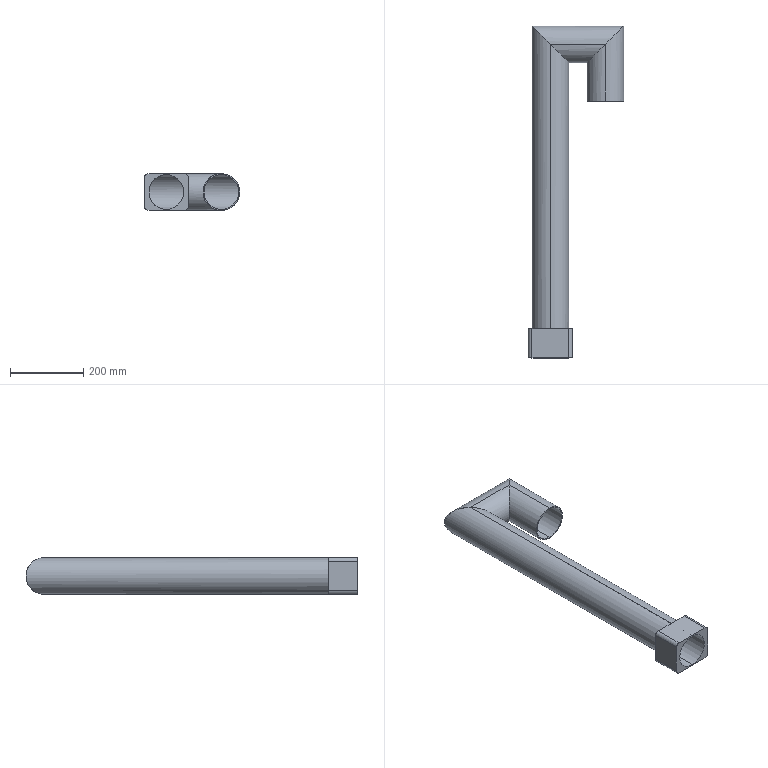Part | STEP file | Water outlet pipe 1 | 1 solid | 24 faces | box 260 x 905 x 100 mm | volume 1213100 mm3 | cylinder 16 | plane 8 | commonest cylinder face diameters 95 x6 100 x6 20 x4